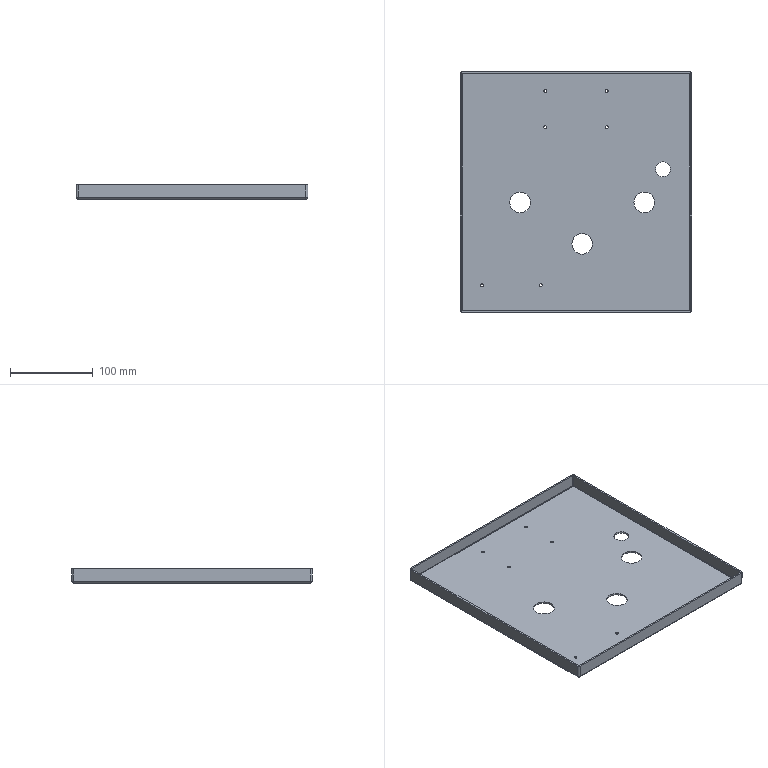Part | SolidWorks | features ICE 17, MoveFace 7, Fillet 2, BaseBody 1 | 1 solid | 55 faces | box 280 x 290 x 17.2 mm | volume 191799 mm3 | cylinder 36 | plane 11 | sphere 8 | commonest cylinder face diameters 3.5 x12 0.8 x8 4.8 x8 25 x6 18 x2